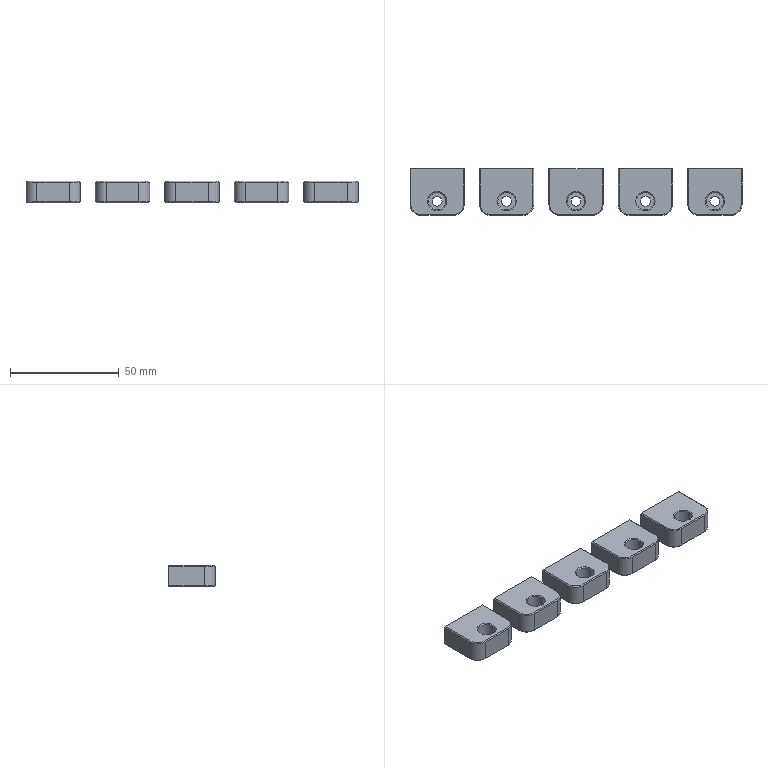Part | 5 solids | 185 faces | box 153 x 21.5 x 10 mm | volume 23349 mm3 | plane 75 | cone 60 | cylinder 50 | commonest cylinder face diameters 3.5 x20 4.5 x10 8.05 x10 10 x10